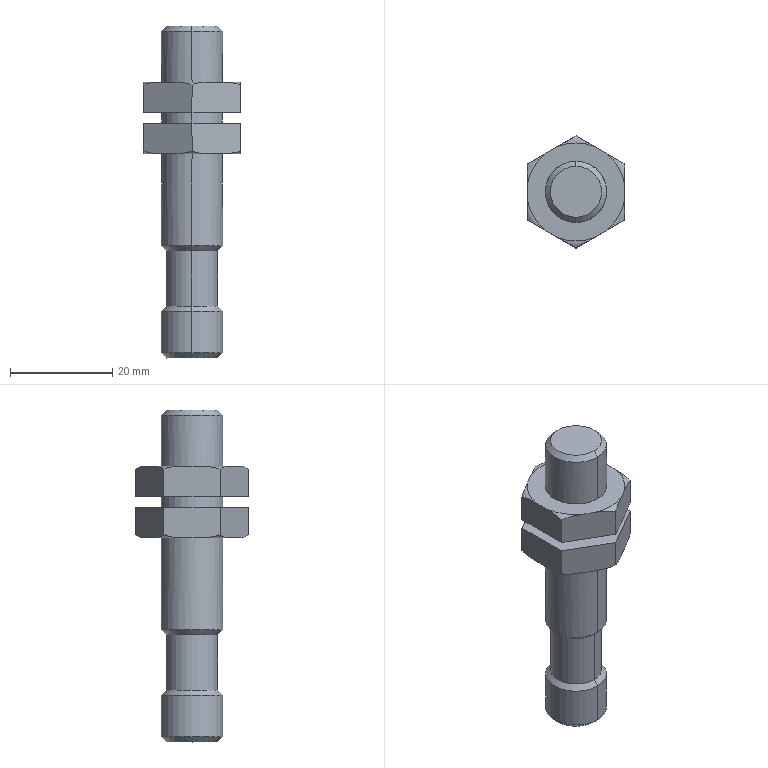Part | NX | features 20 2 | 1 solid | 48 faces | box 19 x 21.939 x 65 mm | volume 9295 mm3 | plane 18 | torus 12 | cylinder 10 | cone 8 | commonest cylinder face diameters 12 x8 10 x2